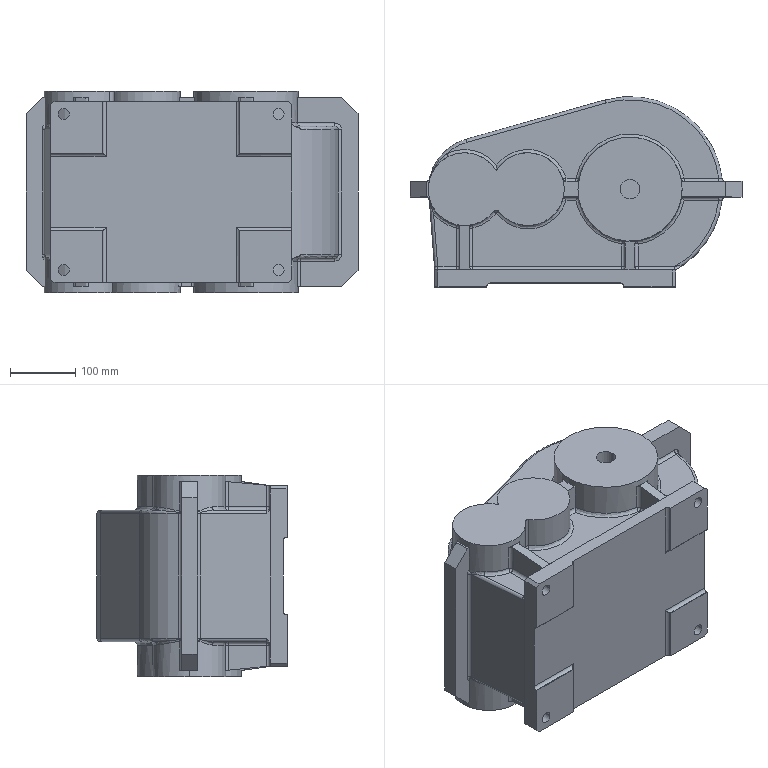Part | SolidWorks | features BaseBody 1 | 1 solid | 237 faces | box 510 x 292.394 x 310 mm | volume 26978776 mm3 | cylinder 90 | plane 83 | spline 64 | commonest cylinder face diameters 10 x65 17 x8 112 x6 160 x5 30 x4 284.788 x2